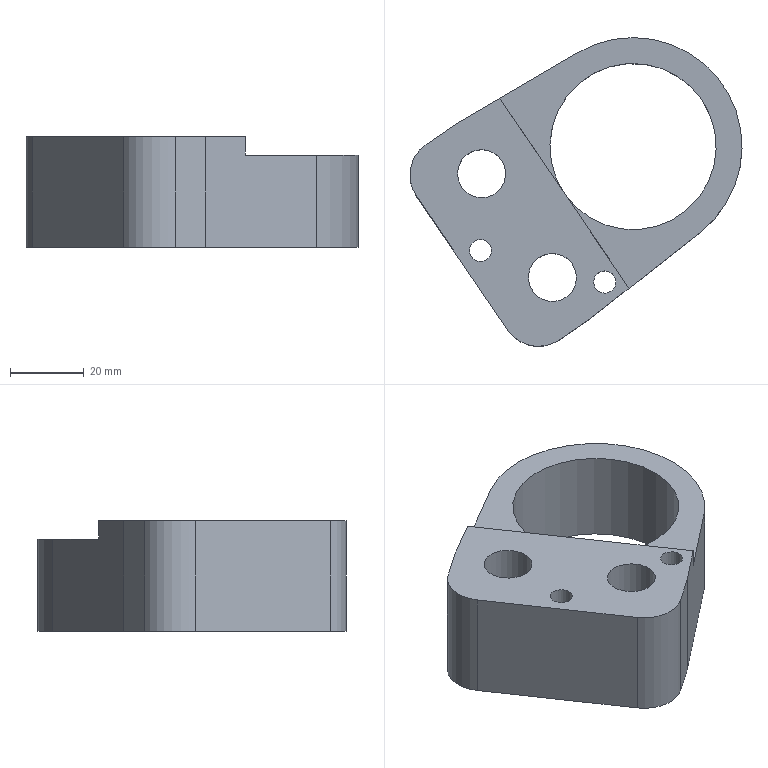Part | NX | features solid 2 | 1 solid | 25 faces | box 89.902 x 83.584 x 30 mm | volume 76435 mm3 | plane 13 | cylinder 12 | commonest cylinder face diameters 6 x2 8 x2 13 x2 19 x2 20 x2 45 x1
STEP:
#1=CARTESIAN_POINT('',(-178.59,-25.771,115.));
#2=VERTEX_POINT('',#1);
#3=CARTESIAN_POINT('',(-178.59,-25.771,110.));
#4=VERTEX_POINT('',#3);
#5=CARTESIAN_POINT('',(-178.59,-25.771,115.));
#6=DIRECTION('',(0.,0.,-1.));
#7=VECTOR('',#6,1000.);
#8=LINE('',#5,#7);
#9=EDGE_CURVE('',#2,#4,#8,.T.);
#10=ORIENTED_EDGE('',*,*,#9,.F.);
#11=CARTESIAN_POINT('',(-189.232,-34.128,115.));
#12=VERTEX_POINT('',#11);
#13=CARTESIAN_POINT('',(-189.232,-34.128,115.));
#14=DIRECTION('',(0.7865,0.6176,0.));
#15=VECTOR('',#14,1000.);
#16=LINE('',#13,#15);
#17=EDGE_CURVE('',#12,#2,#16,.T.);
#18=ORIENTED_EDGE('',*,*,#17,.F.);
#19=CARTESIAN_POINT('',(-189.232,-34.128,85.));
#20=VERTEX_POINT('',#19);
#21=CARTESIAN_POINT('',(-189.232,-34.128,115.));
#22=DIRECTION('',(0.,0.,-1.));
#23=VECTOR('',#22,1000.);
#24=LINE('',#21,#23);
#25=EDGE_CURVE('',#12,#20,#24,.T.);
#26=ORIENTED_EDGE('',*,*,#25,.T.);
#27=CARTESIAN_POINT('',(-159.285,-10.613,85.));
#28=VERTEX_POINT('',#27);
#29=CARTESIAN_POINT('',(-189.232,-34.128,85.));
#30=DIRECTION('',(0.7865,0.6176,0.));
#31=VECTOR('',#30,1000.);
#32=LINE('',#29,#31);
#33=EDGE_CURVE('',#20,#28,#32,.T.);
#34=ORIENTED_EDGE('',*,*,#33,.T.);
#35=CARTESIAN_POINT('',(-159.285,-10.613,110.));
#36=VERTEX_POINT('',#35);
#37=CARTESIAN_POINT('',(-159.285,-10.613,115.));
#38=DIRECTION('',(0.,0.,-1.));
#39=VECTOR('',#38,1000.);
#40=LINE('',#37,#39);
#41=EDGE_CURVE('',#36,#28,#40,.T.);
#42=ORIENTED_EDGE('',*,*,#41,.F.);
#43=CARTESIAN_POINT('',(-189.232,-34.128,110.));
#44=DIRECTION('',(0.7865,0.6176,0.));
#45=VECTOR('',#44,1000.);
#46=LINE('',#43,#45);
#47=EDGE_CURVE('',#4,#36,#46,.T.);
#48=ORIENTED_EDGE('',*,*,#47,.F.);
#49=EDGE_LOOP('',(#10,#18,#26,#34,#42,#48));
#50=FACE_BOUND('',#49,.T.);
#51=CARTESIAN_POINT('',(-189.232,-34.128,115.));
#52=DIRECTION('',(-0.6176,0.7865,0.));
#53=DIRECTION('',(0.7865,0.6176,0.));
#54=AXIS2_PLACEMENT_3D('',#51,#52,#53);
#55=PLANE('',#54);
#56=ADVANCED_FACE('',(#50),#55,.F.);
#57=CARTESIAN_POINT('',(-192.435,38.031,110.));
#58=VERTEX_POINT('',#57);
#59=CARTESIAN_POINT('',(-192.435,38.031,85.));
#60=VERTEX_POINT('',#59);
#61=CARTESIAN_POINT('',(-192.435,38.031,115.));
#62=DIRECTION('',(0.,0.,-1.));
#63=VECTOR('',#62,1000.);
#64=LINE('',#61,#63);
#65=EDGE_CURVE('',#58,#60,#64,.T.);
#66=ORIENTED_EDGE('',*,*,#65,.F.);
#67=CARTESIAN_POINT('',(-177.504,12.589,110.));
#68=DIRECTION('',(0.,0.,-1.));
#69=DIRECTION('',(-0.8264,-0.5631,0.));
#70=AXIS2_PLACEMENT_3D('',#67,#68,#69);
#71=CIRCLE('',#70,29.5);
#72=EDGE_CURVE('',#58,#36,#71,.T.);
#73=ORIENTED_EDGE('',*,*,#72,.T.);
#74=ORIENTED_EDGE('',*,*,#41,.T.);
#75=CARTESIAN_POINT('',(-177.504,12.589,85.));
#76=DIRECTION('',(0.,0.,-1.));
#77=DIRECTION('',(-0.8264,-0.5631,0.));
#78=AXIS2_PLACEMENT_3D('',#75,#76,#77);
#79=CIRCLE('',#78,29.5);
#80=EDGE_CURVE('',#60,#28,#79,.T.);
#81=ORIENTED_EDGE('',*,*,#80,.F.);
#82=EDGE_LOOP('',(#66,#73,#74,#81));
#83=FACE_BOUND('',#82,.T.);
#84=CARTESIAN_POINT('',(-177.504,12.589,115.));
#85=DIRECTION('',(0.,0.,-1.));
#86=DIRECTION('',(-0.8264,-0.5631,0.));
#87=AXIS2_PLACEMENT_3D('',#84,#85,#86);
#88=CYLINDRICAL_SURFACE('',#87,29.5);
#89=ADVANCED_FACE('',(#83),#88,.T.);
#90=CARTESIAN_POINT('',(-225.273,18.76,115.));
#91=VERTEX_POINT('',#90);
#92=CARTESIAN_POINT('',(-213.604,25.608,115.));
#93=VERTEX_POINT('',#92);
#94=CARTESIAN_POINT('',(-225.273,18.76,115.));
#95=DIRECTION('',(0.8624,0.5061,0.));
#96=VECTOR('',#95,1000.);
#97=LINE('',#94,#96);
#98=EDGE_CURVE('',#91,#93,#97,.T.);
#99=ORIENTED_EDGE('',*,*,#98,.T.);
#100=CARTESIAN_POINT('',(-213.604,25.608,110.));
#101=VERTEX_POINT('',#100);
#102=CARTESIAN_POINT('',(-213.604,25.608,115.));
#103=DIRECTION('',(0.,0.,-1.));
#104=VECTOR('',#103,1000.);
#105=LINE('',#102,#104);
#106=EDGE_CURVE('',#93,#101,#105,.T.);
#107=ORIENTED_EDGE('',*,*,#106,.T.);
#108=CARTESIAN_POINT('',(-225.273,18.76,110.));
#109=DIRECTION('',(0.8624,0.5061,0.));
#110=VECTOR('',#109,1000.);
#111=LINE('',#108,#110);
#112=EDGE_CURVE('',#101,#58,#111,.T.);
#113=ORIENTED_EDGE('',*,*,#112,.T.);
#114=ORIENTED_EDGE('',*,*,#65,.T.);
#115=CARTESIAN_POINT('',(-225.273,18.76,85.));
#116=VERTEX_POINT('',#115);
#117=CARTESIAN_POINT('',(-225.273,18.76,85.));
#118=DIRECTION('',(0.8624,0.5061,0.));
#119=VECTOR('',#118,1000.);
#120=LINE('',#117,#119);
#121=EDGE_CURVE('',#116,#60,#120,.T.);
#122=ORIENTED_EDGE('',*,*,#121,.F.);
#123=CARTESIAN_POINT('',(-225.273,18.76,115.));
#124=DIRECTION('',(0.,0.,-1.));
#125=VECTOR('',#124,1000.);
#126=LINE('',#123,#125);
#127=EDGE_CURVE('',#91,#116,#126,.T.);
#128=ORIENTED_EDGE('',*,*,#127,.F.);
#129=EDGE_LOOP('',(#99,#107,#113,#114,#122,#128));
#130=FACE_BOUND('',#129,.T.);
#131=CARTESIAN_POINT('',(-225.273,18.76,115.));
#132=DIRECTION('',(-0.5061,0.8624,0.));
#133=DIRECTION('',(0.8624,0.5061,0.));
#134=AXIS2_PLACEMENT_3D('',#131,#132,#133);
#135=PLANE('',#134);
#136=ADVANCED_FACE('',(#130),#135,.T.);
#137=CARTESIAN_POINT('',(-196.097,-0.08154,85.));
#138=VERTEX_POINT('',#137);
#139=CARTESIAN_POINT('',(-177.504,12.589,85.));
#140=DIRECTION('',(0.,0.,-1.));
#141=DIRECTION('',(-0.8264,-0.5631,0.));
#142=AXIS2_PLACEMENT_3D('',#139,#140,#141);
#143=CIRCLE('',#142,22.5);
#144=EDGE_CURVE('',#138,#138,#143,.T.);
#145=ORIENTED_EDGE('',*,*,#144,.T.);
#146=EDGE_LOOP('',(#145));
#147=FACE_BOUND('',#146,.T.);
#148=CARTESIAN_POINT('',(-196.097,-0.08154,110.));
#149=VERTEX_POINT('',#148);
#150=CARTESIAN_POINT('',(-177.504,12.589,110.));
#151=DIRECTION('',(0.,0.,1.));
#152=DIRECTION('',(0.8264,0.5631,0.));
#153=AXIS2_PLACEMENT_3D('',#150,#151,#152);
#154=CIRCLE('',#153,22.5);
#155=EDGE_CURVE('',#149,#149,#154,.F.);
#156=ORIENTED_EDGE('',*,*,#155,.F.);
#157=EDGE_LOOP('',(#156));
#158=FACE_BOUND('',#157,.T.);
#159=CARTESIAN_POINT('',(-177.504,12.589,115.));
#160=DIRECTION('',(0.,0.,-1.));
#161=DIRECTION('',(-0.8264,-0.5631,0.));
#162=AXIS2_PLACEMENT_3D('',#159,#160,#161);
#163=CYLINDRICAL_SURFACE('',#162,22.5);
#164=ADVANCED_FACE('',(#147,#158),#163,.F.);
#165=CARTESIAN_POINT('',(-204.703,-26.519,115.));
#166=VERTEX_POINT('',#165);
#167=CARTESIAN_POINT('',(-199.332,-22.858,115.));
#168=DIRECTION('',(0.,0.,-1.));
#169=DIRECTION('',(-0.8264,-0.5631,0.));
#170=AXIS2_PLACEMENT_3D('',#167,#168,#169);
#171=CIRCLE('',#170,6.5);
#172=EDGE_CURVE('',#166,#166,#171,.T.);
#173=ORIENTED_EDGE('',*,*,#172,.T.);
#174=EDGE_LOOP('',(#173));
#175=FACE_BOUND('',#174,.T.);
#176=CARTESIAN_POINT('',(-187.653,-25.79,115.));
#177=VERTEX_POINT('',#176);
#178=CARTESIAN_POINT('',(-185.174,-24.101,115.));
#179=DIRECTION('',(0.,0.,-1.));
#180=DIRECTION('',(-0.8264,-0.5631,0.));
#181=AXIS2_PLACEMENT_3D('',#178,#179,#180);
#182=CIRCLE('',#181,3.);
#183=EDGE_CURVE('',#177,#177,#182,.T.);
#184=ORIENTED_EDGE('',*,*,#183,.T.);
#185=EDGE_LOOP('',(#184));
#186=FACE_BOUND('',#185,.T.);
#187=CARTESIAN_POINT('',(-221.301,-17.257,115.));
#188=VERTEX_POINT('',#187);
#189=CARTESIAN_POINT('',(-218.822,-15.568,115.));
#190=DIRECTION('',(0.,0.,-1.));
#191=DIRECTION('',(-0.8264,-0.5631,0.));
#192=AXIS2_PLACEMENT_3D('',#189,#190,#191);
#193=CIRCLE('',#192,3.);
#194=EDGE_CURVE('',#188,#188,#193,.T.);
#195=ORIENTED_EDGE('',*,*,#194,.T.);
#196=EDGE_LOOP('',(#195));
#197=FACE_BOUND('',#196,.T.);
#198=CARTESIAN_POINT('',(-223.85,1.578,115.));
#199=VERTEX_POINT('',#198);
#200=CARTESIAN_POINT('',(-218.479,5.238,115.));
#201=DIRECTION('',(0.,0.,-1.));
#202=DIRECTION('',(-0.8264,-0.5631,0.));
#203=AXIS2_PLACEMENT_3D('',#200,#201,#202);
#204=CIRCLE('',#203,6.5);
#205=EDGE_CURVE('',#199,#199,#204,.T.);
#206=ORIENTED_EDGE('',*,*,#205,.T.);
#207=EDGE_LOOP('',(#206));
#208=FACE_BOUND('',#207,.T.);
#209=CARTESIAN_POINT('',(-233.537,13.128,115.));
#210=VERTEX_POINT('',#209);
#211=CARTESIAN_POINT('',(-241.8,7.497,115.));
#212=DIRECTION('',(0.8264,0.5631,0.));
#213=VECTOR('',#212,1000.);
#214=LINE('',#211,#213);
#215=EDGE_CURVE('',#210,#91,#214,.T.);
#216=ORIENTED_EDGE('',*,*,#215,.F.);
#217=CARTESIAN_POINT('',(-236.169,-0.7668,115.));
#218=VERTEX_POINT('',#217);
#219=CARTESIAN_POINT('',(-227.905,4.865,115.));
#220=DIRECTION('',(0.,0.,-1.));
#221=DIRECTION('',(-0.8264,-0.5631,0.));
#222=AXIS2_PLACEMENT_3D('',#219,#220,#221);
#223=CIRCLE('',#222,10.);
#224=EDGE_CURVE('',#210,#218,#223,.F.);
#225=ORIENTED_EDGE('',*,*,#224,.T.);
#226=CARTESIAN_POINT('',(-211.391,-37.127,115.));
#227=VERTEX_POINT('',#226);
#228=CARTESIAN_POINT('',(-205.76,-45.39,115.));
#229=DIRECTION('',(-0.5631,0.8264,0.));
#230=VECTOR('',#229,1000.);
#231=LINE('',#228,#230);
#232=EDGE_CURVE('',#227,#218,#231,.T.);
#233=ORIENTED_EDGE('',*,*,#232,.F.);
#234=CARTESIAN_POINT('',(-197.496,-39.759,115.));
#235=VERTEX_POINT('',#234);
#236=CARTESIAN_POINT('',(-203.127,-31.495,115.));
#237=DIRECTION('',(0.,0.,-1.));
#238=DIRECTION('',(-0.8264,-0.5631,0.));
#239=AXIS2_PLACEMENT_3D('',#236,#237,#238);
#240=CIRCLE('',#239,10.);
#241=EDGE_CURVE('',#227,#235,#240,.F.);
#242=ORIENTED_EDGE('',*,*,#241,.T.);
#243=CARTESIAN_POINT('',(-189.232,-34.128,115.));
#244=DIRECTION('',(-0.8264,-0.5631,0.));
#245=VECTOR('',#244,1000.);
#246=LINE('',#243,#245);
#247=EDGE_CURVE('',#12,#235,#246,.T.);
#248=ORIENTED_EDGE('',*,*,#247,.F.);
#249=ORIENTED_EDGE('',*,*,#17,.T.);
#250=CARTESIAN_POINT('',(-196.097,-0.08154,115.));
#251=DIRECTION('',(0.5631,-0.8264,0.));
#252=VECTOR('',#251,1000.);
#253=LINE('',#250,#252);
#254=EDGE_CURVE('',#93,#2,#253,.T.);
#255=ORIENTED_EDGE('',*,*,#254,.F.);
#256=ORIENTED_EDGE('',*,*,#98,.F.);
#257=EDGE_LOOP('',(#216,#225,#233,#242,#248,#249,#255,#256));
#258=FACE_BOUND('',#257,.T.);
#259=CARTESIAN_POINT('',(-177.504,12.589,115.));
#260=DIRECTION('',(0.,0.,-1.));
#261=DIRECTION('',(-0.8264,-0.5631,0.));
#262=AXIS2_PLACEMENT_3D('',#259,#260,#261);
#263=PLANE('',#262);
#264=ADVANCED_FACE('',(#175,#186,#197,#208,#258),#263,.F.);
#265=ORIENTED_EDGE('',*,*,#183,.F.);
#266=EDGE_LOOP('',(#265));
#267=FACE_BOUND('',#266,.T.);
#268=CARTESIAN_POINT('',(-187.653,-25.79,105.));
#269=VERTEX_POINT('',#268);
#270=CARTESIAN_POINT('',(-185.174,-24.101,105.));
#271=DIRECTION('',(0.,0.,-1.));
#272=DIRECTION('',(-0.8264,-0.5631,0.));
#273=AXIS2_PLACEMENT_3D('',#270,#271,#272);
#274=CIRCLE('',#273,3.);
#275=EDGE_CURVE('',#269,#269,#274,.F.);
#276=ORIENTED_EDGE('',*,*,#275,.F.);
#277=EDGE_LOOP('',(#276));
#278=FACE_BOUND('',#277,.T.);
#279=CARTESIAN_POINT('',(-185.174,-24.101,115.));
#280=DIRECTION('',(0.,0.,-1.));
#281=DIRECTION('',(-0.8264,-0.5631,0.));
#282=AXIS2_PLACEMENT_3D('',#279,#280,#281);
#283=CYLINDRICAL_SURFACE('',#282,3.);
#284=ADVANCED_FACE('',(#267,#278),#283,.F.);
#285=ORIENTED_EDGE('',*,*,#194,.F.);
#286=EDGE_LOOP('',(#285));
#287=FACE_BOUND('',#286,.T.);
#288=CARTESIAN_POINT('',(-221.301,-17.257,105.));
#289=VERTEX_POINT('',#288);
#290=CARTESIAN_POINT('',(-218.822,-15.568,105.));
#291=DIRECTION('',(0.,0.,-1.));
#292=DIRECTION('',(-0.8264,-0.5631,0.));
#293=AXIS2_PLACEMENT_3D('',#290,#291,#292);
#294=CIRCLE('',#293,3.);
#295=EDGE_CURVE('',#289,#289,#294,.F.);
#296=ORIENTED_EDGE('',*,*,#295,.F.);
#297=EDGE_LOOP('',(#296));
#298=FACE_BOUND('',#297,.T.);
#299=CARTESIAN_POINT('',(-218.822,-15.568,115.));
#300=DIRECTION('',(0.,0.,-1.));
#301=DIRECTION('',(-0.8264,-0.5631,0.));
#302=AXIS2_PLACEMENT_3D('',#299,#300,#301);
#303=CYLINDRICAL_SURFACE('',#302,3.);
#304=ADVANCED_FACE('',(#287,#298),#303,.F.);
#305=ORIENTED_EDGE('',*,*,#205,.F.);
#306=EDGE_LOOP('',(#305));
#307=FACE_BOUND('',#306,.T.);
#308=CARTESIAN_POINT('',(-223.85,1.578,99.));
#309=VERTEX_POINT('',#308);
#310=CARTESIAN_POINT('',(-218.479,5.238,99.));
#311=DIRECTION('',(0.,0.,-1.));
#312=DIRECTION('',(-0.8264,-0.5631,0.));
#313=AXIS2_PLACEMENT_3D('',#310,#311,#312);
#314=CIRCLE('',#313,6.5);
#315=EDGE_CURVE('',#309,#309,#314,.F.);
#316=ORIENTED_EDGE('',*,*,#315,.F.);
#317=EDGE_LOOP('',(#316));
#318=FACE_BOUND('',#317,.T.);
#319=CARTESIAN_POINT('',(-218.479,5.238,115.));
#320=DIRECTION('',(0.,0.,-1.));
#321=DIRECTION('',(-0.8264,-0.5631,0.));
#322=AXIS2_PLACEMENT_3D('',#319,#320,#321);
#323=CYLINDRICAL_SURFACE('',#322,6.5);
#324=ADVANCED_FACE('',(#307,#318),#323,.F.);
#325=ORIENTED_EDGE('',*,*,#172,.F.);
#326=EDGE_LOOP('',(#325));
#327=FACE_BOUND('',#326,.T.);
#328=CARTESIAN_POINT('',(-204.703,-26.519,99.));
#329=VERTEX_POINT('',#328);
#330=CARTESIAN_POINT('',(-199.332,-22.858,99.));
#331=DIRECTION('',(0.,0.,-1.));
#332=DIRECTION('',(-0.8264,-0.5631,0.));
#333=AXIS2_PLACEMENT_3D('',#330,#331,#332);
#334=CIRCLE('',#333,6.5);
#335=EDGE_CURVE('',#329,#329,#334,.F.);
#336=ORIENTED_EDGE('',*,*,#335,.F.);
#337=EDGE_LOOP('',(#336));
#338=FACE_BOUND('',#337,.T.);
#339=CARTESIAN_POINT('',(-199.332,-22.858,115.));
#340=DIRECTION('',(0.,0.,-1.));
#341=DIRECTION('',(-0.8264,-0.5631,0.));
#342=AXIS2_PLACEMENT_3D('',#339,#340,#341);
#343=CYLINDRICAL_SURFACE('',#342,6.5);
#344=ADVANCED_FACE('',(#327,#338),#343,.F.);
#345=CARTESIAN_POINT('',(-233.537,13.128,85.));
#346=VERTEX_POINT('',#345);
#347=CARTESIAN_POINT('',(-241.8,7.497,85.));
#348=DIRECTION('',(0.8264,0.5631,0.));
#349=VECTOR('',#348,1000.);
#350=LINE('',#347,#349);
#351=EDGE_CURVE('',#346,#116,#350,.T.);
#352=ORIENTED_EDGE('',*,*,#351,.F.);
#353=CARTESIAN_POINT('',(-233.537,13.128,115.));
#354=DIRECTION('',(0.,0.,-1.));
#355=VECTOR('',#354,1000.);
#356=LINE('',#353,#355);
#357=EDGE_CURVE('',#346,#210,#356,.F.);
#358=ORIENTED_EDGE('',*,*,#357,.T.);
#359=ORIENTED_EDGE('',*,*,#215,.T.);
#360=ORIENTED_EDGE('',*,*,#127,.T.);
#361=EDGE_LOOP('',(#352,#358,#359,#360));
#362=FACE_BOUND('',#361,.T.);
#363=CARTESIAN_POINT('',(-241.8,7.497,115.));
#364=DIRECTION('',(-0.5631,0.8264,0.));
#365=DIRECTION('',(0.,0.,-1.));
#366=AXIS2_PLACEMENT_3D('',#363,#364,#365);
#367=PLANE('',#366);
#368=ADVANCED_FACE('',(#362),#367,.T.);
#369=ORIENTED_EDGE('',*,*,#232,.T.);
#370=CARTESIAN_POINT('',(-236.169,-0.7668,85.));
#371=VERTEX_POINT('',#370);
#372=CARTESIAN_POINT('',(-236.169,-0.7668,115.));
#373=DIRECTION('',(0.,0.,-1.));
#374=VECTOR('',#373,1000.);
#375=LINE('',#372,#374);
#376=EDGE_CURVE('',#218,#371,#375,.T.);
#377=ORIENTED_EDGE('',*,*,#376,.T.);
#378=CARTESIAN_POINT('',(-211.391,-37.127,85.));
#379=VERTEX_POINT('',#378);
#380=CARTESIAN_POINT('',(-205.76,-45.39,85.));
#381=DIRECTION('',(-0.5631,0.8264,0.));
#382=VECTOR('',#381,1000.);
#383=LINE('',#380,#382);
#384=EDGE_CURVE('',#379,#371,#383,.T.);
#385=ORIENTED_EDGE('',*,*,#384,.F.);
#386=CARTESIAN_POINT('',(-211.391,-37.127,115.));
#387=DIRECTION('',(0.,0.,-1.));
#388=VECTOR('',#387,1000.);
#389=LINE('',#386,#388);
#390=EDGE_CURVE('',#379,#227,#389,.F.);
#391=ORIENTED_EDGE('',*,*,#390,.T.);
#392=EDGE_LOOP('',(#369,#377,#385,#391));
#393=FACE_BOUND('',#392,.T.);
#394=CARTESIAN_POINT('',(-205.76,-45.39,115.));
#395=DIRECTION('',(-0.8264,-0.5631,0.));
#396=DIRECTION('',(0.,0.,1.));
#397=AXIS2_PLACEMENT_3D('',#394,#395,#396);
#398=PLANE('',#397);
#399=ADVANCED_FACE('',(#393),#398,.T.);
#400=ORIENTED_EDGE('',*,*,#247,.T.);
#401=CARTESIAN_POINT('',(-197.496,-39.759,85.));
#402=VERTEX_POINT('',#401);
#403=CARTESIAN_POINT('',(-197.496,-39.759,115.));
#404=DIRECTION('',(0.,0.,-1.));
#405=VECTOR('',#404,1000.);
#406=LINE('',#403,#405);
#407=EDGE_CURVE('',#235,#402,#406,.T.);
#408=ORIENTED_EDGE('',*,*,#407,.T.);
#409=CARTESIAN_POINT('',(-189.232,-34.128,85.));
#410=DIRECTION('',(-0.8264,-0.5631,0.));
#411=VECTOR('',#410,1000.);
#412=LINE('',#409,#411);
#413=EDGE_CURVE('',#20,#402,#412,.T.);
#414=ORIENTED_EDGE('',*,*,#413,.F.);
#415=ORIENTED_EDGE('',*,*,#25,.F.);
#416=EDGE_LOOP('',(#400,#408,#414,#415));
#417=FACE_BOUND('',#416,.T.);
#418=CARTESIAN_POINT('',(-189.232,-34.128,115.));
#419=DIRECTION('',(0.5631,-0.8264,0.));
#420=DIRECTION('',(0.,0.,1.));
#421=AXIS2_PLACEMENT_3D('',#418,#419,#420);
#422=PLANE('',#421);
#423=ADVANCED_FACE('',(#417),#422,.T.);
#424=CARTESIAN_POINT('',(-188.479,-26.354,85.));
#425=VERTEX_POINT('',#424);
#426=CARTESIAN_POINT('',(-185.174,-24.101,85.));
#427=DIRECTION('',(0.,0.,-1.));
#428=DIRECTION('',(-0.8264,-0.5631,0.));
#429=AXIS2_PLACEMENT_3D('',#426,#427,#428);
#430=CIRCLE('',#429,4.);
#431=EDGE_CURVE('',#425,#425,#430,.T.);
#432=ORIENTED_EDGE('',*,*,#431,.F.);
#433=EDGE_LOOP('',(#432));
#434=FACE_BOUND('',#433,.T.);
#435=CARTESIAN_POINT('',(-222.127,-17.82,85.));
#436=VERTEX_POINT('',#435);
#437=CARTESIAN_POINT('',(-218.822,-15.568,85.));
#438=DIRECTION('',(0.,0.,-1.));
#439=DIRECTION('',(-0.8264,-0.5631,0.));
#440=AXIS2_PLACEMENT_3D('',#437,#438,#439);
#441=CIRCLE('',#440,4.);
#442=EDGE_CURVE('',#436,#436,#441,.T.);
#443=ORIENTED_EDGE('',*,*,#442,.F.);
#444=EDGE_LOOP('',(#443));
#445=FACE_BOUND('',#444,.T.);
#446=CARTESIAN_POINT('',(-226.329,-0.1119,85.));
#447=VERTEX_POINT('',#446);
#448=CARTESIAN_POINT('',(-218.479,5.238,85.));
#449=DIRECTION('',(0.,0.,-1.));
#450=DIRECTION('',(-0.8264,-0.5631,0.));
#451=AXIS2_PLACEMENT_3D('',#448,#449,#450);
#452=CIRCLE('',#451,9.5);
#453=EDGE_CURVE('',#447,#447,#452,.T.);
#454=ORIENTED_EDGE('',*,*,#453,.F.);
#455=EDGE_LOOP('',(#454));
#456=FACE_BOUND('',#455,.T.);
#457=CARTESIAN_POINT('',(-207.183,-28.208,85.));
#458=VERTEX_POINT('',#457);
#459=CARTESIAN_POINT('',(-199.332,-22.858,85.));
#460=DIRECTION('',(0.,0.,-1.));
#461=DIRECTION('',(-0.8264,-0.5631,0.));
#462=AXIS2_PLACEMENT_3D('',#459,#460,#461);
#463=CIRCLE('',#462,9.5);
#464=EDGE_CURVE('',#458,#458,#463,.T.);
#465=ORIENTED_EDGE('',*,*,#464,.F.);
#466=EDGE_LOOP('',(#465));
#467=FACE_BOUND('',#466,.T.);
#468=ORIENTED_EDGE('',*,*,#384,.T.);
#469=CARTESIAN_POINT('',(-227.905,4.865,85.));
#470=DIRECTION('',(0.,0.,-1.));
#471=DIRECTION('',(-0.8264,-0.5631,0.));
#472=AXIS2_PLACEMENT_3D('',#469,#470,#471);
#473=CIRCLE('',#472,10.);
#474=EDGE_CURVE('',#371,#346,#473,.T.);
#475=ORIENTED_EDGE('',*,*,#474,.T.);
#476=ORIENTED_EDGE('',*,*,#351,.T.);
#477=ORIENTED_EDGE('',*,*,#121,.T.);
#478=ORIENTED_EDGE('',*,*,#80,.T.);
#479=ORIENTED_EDGE('',*,*,#33,.F.);
#480=ORIENTED_EDGE('',*,*,#413,.T.);
#481=CARTESIAN_POINT('',(-203.127,-31.495,85.));
#482=DIRECTION('',(0.,0.,-1.));
#483=DIRECTION('',(-0.8264,-0.5631,0.));
#484=AXIS2_PLACEMENT_3D('',#481,#482,#483);
#485=CIRCLE('',#484,10.);
#486=EDGE_CURVE('',#402,#379,#485,.T.);
#487=ORIENTED_EDGE('',*,*,#486,.T.);
#488=EDGE_LOOP('',(#468,#475,#476,#477,#478,#479,#480,#487));
#489=FACE_BOUND('',#488,.T.);
#490=ORIENTED_EDGE('',*,*,#144,.F.);
#491=EDGE_LOOP('',(#490));
#492=FACE_BOUND('',#491,.T.);
#493=CARTESIAN_POINT('',(-177.504,12.589,85.));
#494=DIRECTION('',(0.,0.,-1.));
#495=DIRECTION('',(-0.8264,-0.5631,0.));
#496=AXIS2_PLACEMENT_3D('',#493,#494,#495);
#497=PLANE('',#496);
#498=ADVANCED_FACE('',(#434,#445,#456,#467,#489,#492),#497,.T.);
#499=CARTESIAN_POINT('',(-207.183,-28.208,99.));
#500=VERTEX_POINT('',#499);
#501=CARTESIAN_POINT('',(-199.332,-22.858,99.));
#502=DIRECTION('',(0.,0.,-1.));
#503=DIRECTION('',(-0.8264,-0.5631,0.));
#504=AXIS2_PLACEMENT_3D('',#501,#502,#503);
#505=CIRCLE('',#504,9.5);
#506=EDGE_CURVE('',#500,#500,#505,.T.);
#507=ORIENTED_EDGE('',*,*,#506,.T.);
#508=EDGE_LOOP('',(#507));
#509=FACE_BOUND('',#508,.T.);
#510=ORIENTED_EDGE('',*,*,#335,.T.);
#511=EDGE_LOOP('',(#510));
#512=FACE_BOUND('',#511,.T.);
#513=CARTESIAN_POINT('',(-199.332,-22.858,99.));
#514=DIRECTION('',(0.,0.,-1.));
#515=DIRECTION('',(-0.8264,-0.5631,0.));
#516=AXIS2_PLACEMENT_3D('',#513,#514,#515);
#517=PLANE('',#516);
#518=ADVANCED_FACE('',(#509,#512),#517,.T.);
#519=ORIENTED_EDGE('',*,*,#506,.F.);
#520=EDGE_LOOP('',(#519));
#521=FACE_BOUND('',#520,.T.);
#522=ORIENTED_EDGE('',*,*,#464,.T.);
#523=EDGE_LOOP('',(#522));
#524=FACE_BOUND('',#523,.T.);
#525=CARTESIAN_POINT('',(-199.332,-22.858,99.));
#526=DIRECTION('',(0.,0.,-1.));
#527=DIRECTION('',(-0.8264,-0.5631,0.));
#528=AXIS2_PLACEMENT_3D('',#525,#526,#527);
#529=CYLINDRICAL_SURFACE('',#528,9.5);
#530=ADVANCED_FACE('',(#521,#524),#529,.F.);
#531=CARTESIAN_POINT('',(-226.329,-0.1119,99.));
#532=VERTEX_POINT('',#531);
#533=CARTESIAN_POINT('',(-218.479,5.238,99.));
#534=DIRECTION('',(0.,0.,-1.));
#535=DIRECTION('',(-0.8264,-0.5631,0.));
#536=AXIS2_PLACEMENT_3D('',#533,#534,#535);
#537=CIRCLE('',#536,9.5);
#538=EDGE_CURVE('',#532,#532,#537,.T.);
#539=ORIENTED_EDGE('',*,*,#538,.T.);
#540=EDGE_LOOP('',(#539));
#541=FACE_BOUND('',#540,.T.);
#542=ORIENTED_EDGE('',*,*,#315,.T.);
#543=EDGE_LOOP('',(#542));
#544=FACE_BOUND('',#543,.T.);
#545=CARTESIAN_POINT('',(-218.479,5.238,99.));
#546=DIRECTION('',(0.,0.,-1.));
#547=DIRECTION('',(-0.8264,-0.5631,0.));
#548=AXIS2_PLACEMENT_3D('',#545,#546,#547);
#549=PLANE('',#548);
#550=ADVANCED_FACE('',(#541,#544),#549,.T.);
#551=ORIENTED_EDGE('',*,*,#538,.F.);
#552=EDGE_LOOP('',(#551));
#553=FACE_BOUND('',#552,.T.);
#554=ORIENTED_EDGE('',*,*,#453,.T.);
#555=EDGE_LOOP('',(#554));
#556=FACE_BOUND('',#555,.T.);
#557=CARTESIAN_POINT('',(-218.479,5.238,99.));
#558=DIRECTION('',(0.,0.,-1.));
#559=DIRECTION('',(-0.8264,-0.5631,0.));
#560=AXIS2_PLACEMENT_3D('',#557,#558,#559);
#561=CYLINDRICAL_SURFACE('',#560,9.5);
#562=ADVANCED_FACE('',(#553,#556),#561,.F.);
#563=CARTESIAN_POINT('',(-222.127,-17.82,105.));
#564=VERTEX_POINT('',#563);
#565=CARTESIAN_POINT('',(-218.822,-15.568,105.));
#566=DIRECTION('',(0.,0.,-1.));
#567=DIRECTION('',(-0.8264,-0.5631,0.));
#568=AXIS2_PLACEMENT_3D('',#565,#566,#567);
#569=CIRCLE('',#568,4.);
#570=EDGE_CURVE('',#564,#564,#569,.T.);
#571=ORIENTED_EDGE('',*,*,#570,.T.);
#572=EDGE_LOOP('',(#571));
#573=FACE_BOUND('',#572,.T.);
#574=ORIENTED_EDGE('',*,*,#295,.T.);
#575=EDGE_LOOP('',(#574));
#576=FACE_BOUND('',#575,.T.);
#577=CARTESIAN_POINT('',(-218.822,-15.568,105.));
#578=DIRECTION('',(0.,0.,-1.));
#579=DIRECTION('',(-0.8264,-0.5631,0.));
#580=AXIS2_PLACEMENT_3D('',#577,#578,#579);
#581=PLANE('',#580);
#582=ADVANCED_FACE('',(#573,#576),#581,.T.);
#583=ORIENTED_EDGE('',*,*,#570,.F.);
#584=EDGE_LOOP('',(#583));
#585=FACE_BOUND('',#584,.T.);
#586=ORIENTED_EDGE('',*,*,#442,.T.);
#587=EDGE_LOOP('',(#586));
#588=FACE_BOUND('',#587,.T.);
#589=CARTESIAN_POINT('',(-218.822,-15.568,105.));
#590=DIRECTION('',(0.,0.,-1.));
#591=DIRECTION('',(-0.8264,-0.5631,0.));
#592=AXIS2_PLACEMENT_3D('',#589,#590,#591);
#593=CYLINDRICAL_SURFACE('',#592,4.);
#594=ADVANCED_FACE('',(#585,#588),#593,.F.);
#595=CARTESIAN_POINT('',(-188.479,-26.354,105.));
#596=VERTEX_POINT('',#595);
#597=CARTESIAN_POINT('',(-185.174,-24.101,105.));
#598=DIRECTION('',(0.,0.,-1.));
#599=DIRECTION('',(-0.8264,-0.5631,0.));
#600=AXIS2_PLACEMENT_3D('',#597,#598,#599);
#601=CIRCLE('',#600,4.);
#602=EDGE_CURVE('',#596,#596,#601,.T.);
#603=ORIENTED_EDGE('',*,*,#602,.T.);
#604=EDGE_LOOP('',(#603));
#605=FACE_BOUND('',#604,.T.);
#606=ORIENTED_EDGE('',*,*,#275,.T.);
#607=EDGE_LOOP('',(#606));
#608=FACE_BOUND('',#607,.T.);
#609=CARTESIAN_POINT('',(-185.174,-24.101,105.));
#610=DIRECTION('',(0.,0.,-1.));
#611=DIRECTION('',(-0.8264,-0.5631,0.));
#612=AXIS2_PLACEMENT_3D('',#609,#610,#611);
#613=PLANE('',#612);
#614=ADVANCED_FACE('',(#605,#608),#613,.T.);
#615=ORIENTED_EDGE('',*,*,#602,.F.);
#616=EDGE_LOOP('',(#615));
#617=FACE_BOUND('',#616,.T.);
#618=ORIENTED_EDGE('',*,*,#431,.T.);
#619=EDGE_LOOP('',(#618));
#620=FACE_BOUND('',#619,.T.);
#621=CARTESIAN_POINT('',(-185.174,-24.101,105.));
#622=DIRECTION('',(0.,0.,-1.));
#623=DIRECTION('',(-0.8264,-0.5631,0.));
#624=AXIS2_PLACEMENT_3D('',#621,#622,#623);
#625=CYLINDRICAL_SURFACE('',#624,4.);
#626=ADVANCED_FACE('',(#617,#620),#625,.F.);
#627=CARTESIAN_POINT('',(-213.604,25.608,110.));
#628=DIRECTION('',(0.5631,-0.8264,0.));
#629=VECTOR('',#628,1000.);
#630=LINE('',#627,#629);
#631=EDGE_CURVE('',#149,#4,#630,.T.);
#632=ORIENTED_EDGE('',*,*,#631,.T.);
#633=ORIENTED_EDGE('',*,*,#47,.T.);
#634=ORIENTED_EDGE('',*,*,#72,.F.);
#635=ORIENTED_EDGE('',*,*,#112,.F.);
#636=CARTESIAN_POINT('',(-213.604,25.608,110.));
#637=DIRECTION('',(0.5631,-0.8264,0.));
#638=VECTOR('',#637,1000.);
#639=LINE('',#636,#638);
#640=EDGE_CURVE('',#101,#149,#639,.T.);
#641=ORIENTED_EDGE('',*,*,#640,.T.);
#642=ORIENTED_EDGE('',*,*,#155,.T.);
#643=EDGE_LOOP('',(#632,#633,#634,#635,#641,#642));
#644=FACE_BOUND('',#643,.T.);
#645=CARTESIAN_POINT('',(-185.926,6.85,110.));
#646=DIRECTION('',(0.,0.,1.));
#647=DIRECTION('',(0.8264,0.5631,0.));
#648=AXIS2_PLACEMENT_3D('',#645,#646,#647);
#649=PLANE('',#648);
#650=ADVANCED_FACE('',(#644),#649,.T.);
#651=ORIENTED_EDGE('',*,*,#631,.F.);
#652=ORIENTED_EDGE('',*,*,#640,.F.);
#653=ORIENTED_EDGE('',*,*,#106,.F.);
#654=ORIENTED_EDGE('',*,*,#254,.T.);
#655=ORIENTED_EDGE('',*,*,#9,.T.);
#656=EDGE_LOOP('',(#651,#652,#653,#654,#655));
#657=FACE_BOUND('',#656,.T.);
#658=CARTESIAN_POINT('',(-213.604,25.608,115.));
#659=DIRECTION('',(0.8264,0.5631,0.));
#660=DIRECTION('',(0.5631,-0.8264,0.));
#661=AXIS2_PLACEMENT_3D('',#658,#659,#660);
#662=PLANE('',#661);
#663=ADVANCED_FACE('',(#657),#662,.T.);
#664=ORIENTED_EDGE('',*,*,#224,.F.);
#665=ORIENTED_EDGE('',*,*,#357,.F.);
#666=ORIENTED_EDGE('',*,*,#474,.F.);
#667=ORIENTED_EDGE('',*,*,#376,.F.);
#668=EDGE_LOOP('',(#664,#665,#666,#667));
#669=FACE_BOUND('',#668,.T.);
#670=CARTESIAN_POINT('',(-227.905,4.865,115.));
#671=DIRECTION('',(0.,0.,-1.));
#672=DIRECTION('',(-0.8264,-0.5631,0.));
#673=AXIS2_PLACEMENT_3D('',#670,#671,#672);
#674=CYLINDRICAL_SURFACE('',#673,10.);
#675=ADVANCED_FACE('',(#669),#674,.T.);
#676=ORIENTED_EDGE('',*,*,#241,.F.);
#677=ORIENTED_EDGE('',*,*,#390,.F.);
#678=ORIENTED_EDGE('',*,*,#486,.F.);
#679=ORIENTED_EDGE('',*,*,#407,.F.);
#680=EDGE_LOOP('',(#676,#677,#678,#679));
#681=FACE_BOUND('',#680,.T.);
#682=CARTESIAN_POINT('',(-203.127,-31.495,115.));
#683=DIRECTION('',(0.,0.,-1.));
#684=DIRECTION('',(-0.8264,-0.5631,0.));
#685=AXIS2_PLACEMENT_3D('',#682,#683,#684);
#686=CYLINDRICAL_SURFACE('',#685,10.);
#687=ADVANCED_FACE('',(#681),#686,.T.);
#688=CLOSED_SHELL('',(#56,#89,#136,#164,#264,#284,#304,#324,#344,#368,#399,#423,#498,#518,#530,#550,#562,#582,#594,#614,#626,#650,#663,#675,#687));
#689=MANIFOLD_SOLID_BREP('',#688);
#690=(LENGTH_UNIT()NAMED_UNIT(*)SI_UNIT(.MILLI.,.METRE.));
#691=UNCERTAINTY_MEASURE_WITH_UNIT(LENGTH_MEASURE(0.00001),#690,'','');
#692=(NAMED_UNIT(*)PLANE_ANGLE_UNIT()SI_UNIT($,.RADIAN.));
#693=(NAMED_UNIT(*)SI_UNIT($,.STERADIAN.)SOLID_ANGLE_UNIT());
#694=(GEOMETRIC_REPRESENTATION_CONTEXT(3)GLOBAL_UNCERTAINTY_ASSIGNED_CONTEXT((#691))GLOBAL_UNIT_ASSIGNED_CONTEXT((#690,#692,#693))REPRESENTATION_CONTEXT('',''));
#695=ADVANCED_BREP_SHAPE_REPRESENTATION('',(#689),#694);